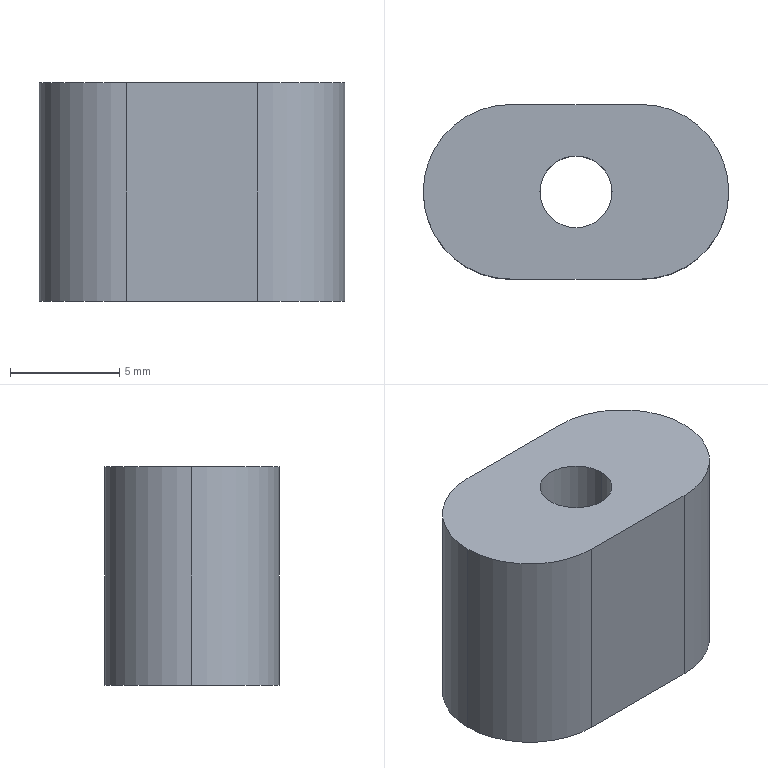Part | STEP file | 09-24 keyboard knob | 1 solid | 10 faces | box 14 x 8 x 10 mm | volume 897.125 mm3 | cylinder 6 | plane 4 | commonest cylinder face diameters 8 x4 3.3 x2
STEP:
#1=CARTESIAN_POINT('',(-1.65,0.,0.));
#2=VERTEX_POINT('',#1);
#3=CARTESIAN_POINT('',(1.65,0.,0.));
#4=VERTEX_POINT('',#3);
#5=CARTESIAN_POINT('',(0.,0.,0.));
#6=DIRECTION('',(0.,0.,1.));
#7=DIRECTION('',(1.,0.,0.));
#8=AXIS2_PLACEMENT_3D('',#5,#6,#7);
#9=CIRCLE('',#8,1.65);
#10=EDGE_CURVE('',#2,#4,#9,.T.);
#11=ORIENTED_EDGE('',*,*,#10,.F.);
#12=CARTESIAN_POINT('',(-1.65,0.,10.));
#13=VERTEX_POINT('',#12);
#14=CARTESIAN_POINT('',(-1.65,0.,10.));
#15=DIRECTION('',(0.,0.,1.));
#16=VECTOR('',#15,1000.);
#17=LINE('',#14,#16);
#18=EDGE_CURVE('',#2,#13,#17,.T.);
#19=ORIENTED_EDGE('',*,*,#18,.T.);
#20=CARTESIAN_POINT('',(1.65,0.,10.));
#21=VERTEX_POINT('',#20);
#22=CARTESIAN_POINT('',(0.,0.,10.));
#23=DIRECTION('',(0.,0.,1.));
#24=DIRECTION('',(1.,0.,0.));
#25=AXIS2_PLACEMENT_3D('',#22,#23,#24);
#26=CIRCLE('',#25,1.65);
#27=EDGE_CURVE('',#13,#21,#26,.T.);
#28=ORIENTED_EDGE('',*,*,#27,.T.);
#29=CARTESIAN_POINT('',(1.65,0.,10.));
#30=DIRECTION('',(0.,0.,1.));
#31=VECTOR('',#30,1000.);
#32=LINE('',#29,#31);
#33=EDGE_CURVE('',#4,#21,#32,.T.);
#34=ORIENTED_EDGE('',*,*,#33,.F.);
#35=EDGE_LOOP('',(#11,#19,#28,#34));
#36=FACE_OUTER_BOUND('',#35,.T.);
#37=CARTESIAN_POINT('',(0.,0.,10.));
#38=DIRECTION('',(0.,0.,1.));
#39=DIRECTION('',(1.,0.,0.));
#40=AXIS2_PLACEMENT_3D('',#37,#38,#39);
#41=CYLINDRICAL_SURFACE('',#40,1.65);
#42=ADVANCED_FACE('',(#36),#41,.F.);
#43=CARTESIAN_POINT('',(3.,4.,10.));
#44=VERTEX_POINT('',#43);
#45=CARTESIAN_POINT('',(-3.,4.,10.));
#46=VERTEX_POINT('',#45);
#47=CARTESIAN_POINT('',(-7.,4.,10.));
#48=DIRECTION('',(-1.,0.,0.));
#49=VECTOR('',#48,1000.);
#50=LINE('',#47,#49);
#51=EDGE_CURVE('',#44,#46,#50,.T.);
#52=ORIENTED_EDGE('',*,*,#51,.F.);
#53=CARTESIAN_POINT('',(3.,4.,0.));
#54=VERTEX_POINT('',#53);
#55=CARTESIAN_POINT('',(3.,4.,10.));
#56=DIRECTION('',(0.,0.,-1.));
#57=VECTOR('',#56,1000.);
#58=LINE('',#55,#57);
#59=EDGE_CURVE('',#44,#54,#58,.T.);
#60=ORIENTED_EDGE('',*,*,#59,.T.);
#61=CARTESIAN_POINT('',(-3.,4.,0.));
#62=VERTEX_POINT('',#61);
#63=CARTESIAN_POINT('',(-7.,4.,0.));
#64=DIRECTION('',(-1.,0.,0.));
#65=VECTOR('',#64,1000.);
#66=LINE('',#63,#65);
#67=EDGE_CURVE('',#54,#62,#66,.T.);
#68=ORIENTED_EDGE('',*,*,#67,.T.);
#69=CARTESIAN_POINT('',(-3.,4.,10.));
#70=DIRECTION('',(0.,0.,1.));
#71=VECTOR('',#70,1000.);
#72=LINE('',#69,#71);
#73=EDGE_CURVE('',#62,#46,#72,.T.);
#74=ORIENTED_EDGE('',*,*,#73,.T.);
#75=EDGE_LOOP('',(#52,#60,#68,#74));
#76=FACE_OUTER_BOUND('',#75,.T.);
#77=CARTESIAN_POINT('',(-7.,4.,10.));
#78=DIRECTION('',(0.,-1.,0.));
#79=DIRECTION('',(0.,0.,-1.));
#80=AXIS2_PLACEMENT_3D('',#77,#78,#79);
#81=PLANE('',#80);
#82=ADVANCED_FACE('',(#76),#81,.F.);
#83=CARTESIAN_POINT('',(-3.,-4.,0.));
#84=VERTEX_POINT('',#83);
#85=CARTESIAN_POINT('',(3.,-4.,0.));
#86=VERTEX_POINT('',#85);
#87=CARTESIAN_POINT('',(-7.,-4.,0.));
#88=DIRECTION('',(1.,0.,0.));
#89=VECTOR('',#88,1000.);
#90=LINE('',#87,#89);
#91=EDGE_CURVE('',#84,#86,#90,.T.);
#92=ORIENTED_EDGE('',*,*,#91,.T.);
#93=CARTESIAN_POINT('',(3.,-4.,10.));
#94=VERTEX_POINT('',#93);
#95=CARTESIAN_POINT('',(3.,-4.,10.));
#96=DIRECTION('',(0.,0.,1.));
#97=VECTOR('',#96,1000.);
#98=LINE('',#95,#97);
#99=EDGE_CURVE('',#86,#94,#98,.T.);
#100=ORIENTED_EDGE('',*,*,#99,.T.);
#101=CARTESIAN_POINT('',(-3.,-4.,10.));
#102=VERTEX_POINT('',#101);
#103=CARTESIAN_POINT('',(-7.,-4.,10.));
#104=DIRECTION('',(1.,0.,0.));
#105=VECTOR('',#104,1000.);
#106=LINE('',#103,#105);
#107=EDGE_CURVE('',#102,#94,#106,.T.);
#108=ORIENTED_EDGE('',*,*,#107,.F.);
#109=CARTESIAN_POINT('',(-3.,-4.,10.));
#110=DIRECTION('',(0.,0.,-1.));
#111=VECTOR('',#110,1000.);
#112=LINE('',#109,#111);
#113=EDGE_CURVE('',#102,#84,#112,.T.);
#114=ORIENTED_EDGE('',*,*,#113,.T.);
#115=EDGE_LOOP('',(#92,#100,#108,#114));
#116=FACE_OUTER_BOUND('',#115,.T.);
#117=CARTESIAN_POINT('',(-7.,-4.,10.));
#118=DIRECTION('',(0.,1.,0.));
#119=DIRECTION('',(0.,0.,1.));
#120=AXIS2_PLACEMENT_3D('',#117,#118,#119);
#121=PLANE('',#120);
#122=ADVANCED_FACE('',(#116),#121,.F.);
#123=CARTESIAN_POINT('',(0.,0.,10.));
#124=DIRECTION('',(0.,0.,1.));
#125=DIRECTION('',(1.,0.,0.));
#126=AXIS2_PLACEMENT_3D('',#123,#124,#125);
#127=CIRCLE('',#126,1.65);
#128=EDGE_CURVE('',#21,#13,#127,.T.);
#129=ORIENTED_EDGE('',*,*,#128,.F.);
#130=ORIENTED_EDGE('',*,*,#27,.F.);
#131=EDGE_LOOP('',(#129,#130));
#132=FACE_BOUND('',#131,.T.);
#133=ORIENTED_EDGE('',*,*,#107,.T.);
#134=CARTESIAN_POINT('',(7.,0.,10.));
#135=VERTEX_POINT('',#134);
#136=CARTESIAN_POINT('',(3.,0.,10.));
#137=DIRECTION('',(0.,0.,1.));
#138=DIRECTION('',(1.,0.,0.));
#139=AXIS2_PLACEMENT_3D('',#136,#137,#138);
#140=CIRCLE('',#139,4.);
#141=EDGE_CURVE('',#94,#135,#140,.T.);
#142=ORIENTED_EDGE('',*,*,#141,.T.);
#143=CARTESIAN_POINT('',(3.,0.,10.));
#144=DIRECTION('',(0.,0.,1.));
#145=DIRECTION('',(1.,0.,0.));
#146=AXIS2_PLACEMENT_3D('',#143,#144,#145);
#147=CIRCLE('',#146,4.);
#148=EDGE_CURVE('',#135,#44,#147,.T.);
#149=ORIENTED_EDGE('',*,*,#148,.T.);
#150=ORIENTED_EDGE('',*,*,#51,.T.);
#151=CARTESIAN_POINT('',(-7.,0.,10.));
#152=VERTEX_POINT('',#151);
#153=CARTESIAN_POINT('',(-3.,0.,10.));
#154=DIRECTION('',(0.,0.,1.));
#155=DIRECTION('',(1.,0.,0.));
#156=AXIS2_PLACEMENT_3D('',#153,#154,#155);
#157=CIRCLE('',#156,4.);
#158=EDGE_CURVE('',#46,#152,#157,.T.);
#159=ORIENTED_EDGE('',*,*,#158,.T.);
#160=CARTESIAN_POINT('',(-3.,0.,10.));
#161=DIRECTION('',(0.,0.,1.));
#162=DIRECTION('',(1.,0.,0.));
#163=AXIS2_PLACEMENT_3D('',#160,#161,#162);
#164=CIRCLE('',#163,4.);
#165=EDGE_CURVE('',#152,#102,#164,.T.);
#166=ORIENTED_EDGE('',*,*,#165,.T.);
#167=EDGE_LOOP('',(#133,#142,#149,#150,#159,#166));
#168=FACE_OUTER_BOUND('',#167,.T.);
#169=CARTESIAN_POINT('',(7.,-4.,10.));
#170=DIRECTION('',(0.,0.,1.));
#171=DIRECTION('',(1.,0.,0.));
#172=AXIS2_PLACEMENT_3D('',#169,#170,#171);
#173=PLANE('',#172);
#174=ADVANCED_FACE('',(#132,#168),#173,.T.);
#175=CARTESIAN_POINT('',(0.,0.,0.));
#176=DIRECTION('',(0.,0.,1.));
#177=DIRECTION('',(1.,0.,0.));
#178=AXIS2_PLACEMENT_3D('',#175,#176,#177);
#179=CIRCLE('',#178,1.65);
#180=EDGE_CURVE('',#4,#2,#179,.T.);
#181=ORIENTED_EDGE('',*,*,#180,.T.);
#182=ORIENTED_EDGE('',*,*,#10,.T.);
#183=EDGE_LOOP('',(#181,#182));
#184=FACE_BOUND('',#183,.T.);
#185=CARTESIAN_POINT('',(7.,0.,0.));
#186=VERTEX_POINT('',#185);
#187=CARTESIAN_POINT('',(3.,0.,0.));
#188=DIRECTION('',(0.,0.,-1.));
#189=DIRECTION('',(1.,0.,0.));
#190=AXIS2_PLACEMENT_3D('',#187,#188,#189);
#191=CIRCLE('',#190,4.);
#192=EDGE_CURVE('',#54,#186,#191,.T.);
#193=ORIENTED_EDGE('',*,*,#192,.T.);
#194=CARTESIAN_POINT('',(3.,0.,0.));
#195=DIRECTION('',(0.,0.,-1.));
#196=DIRECTION('',(1.,0.,0.));
#197=AXIS2_PLACEMENT_3D('',#194,#195,#196);
#198=CIRCLE('',#197,4.);
#199=EDGE_CURVE('',#186,#86,#198,.T.);
#200=ORIENTED_EDGE('',*,*,#199,.T.);
#201=ORIENTED_EDGE('',*,*,#91,.F.);
#202=CARTESIAN_POINT('',(-7.,0.,0.));
#203=VERTEX_POINT('',#202);
#204=CARTESIAN_POINT('',(-3.,0.,0.));
#205=DIRECTION('',(0.,0.,-1.));
#206=DIRECTION('',(1.,0.,0.));
#207=AXIS2_PLACEMENT_3D('',#204,#205,#206);
#208=CIRCLE('',#207,4.);
#209=EDGE_CURVE('',#84,#203,#208,.T.);
#210=ORIENTED_EDGE('',*,*,#209,.T.);
#211=CARTESIAN_POINT('',(-3.,0.,0.));
#212=DIRECTION('',(0.,0.,-1.));
#213=DIRECTION('',(1.,0.,0.));
#214=AXIS2_PLACEMENT_3D('',#211,#212,#213);
#215=CIRCLE('',#214,4.);
#216=EDGE_CURVE('',#203,#62,#215,.T.);
#217=ORIENTED_EDGE('',*,*,#216,.T.);
#218=ORIENTED_EDGE('',*,*,#67,.F.);
#219=EDGE_LOOP('',(#193,#200,#201,#210,#217,#218));
#220=FACE_OUTER_BOUND('',#219,.T.);
#221=CARTESIAN_POINT('',(7.,-4.,0.));
#222=DIRECTION('',(0.,0.,1.));
#223=DIRECTION('',(1.,0.,0.));
#224=AXIS2_PLACEMENT_3D('',#221,#222,#223);
#225=PLANE('',#224);
#226=ADVANCED_FACE('',(#184,#220),#225,.F.);
#227=ORIENTED_EDGE('',*,*,#59,.F.);
#228=ORIENTED_EDGE('',*,*,#148,.F.);
#229=CARTESIAN_POINT('',(7.,0.,10.));
#230=DIRECTION('',(0.,0.,1.));
#231=VECTOR('',#230,1000.);
#232=LINE('',#229,#231);
#233=EDGE_CURVE('',#186,#135,#232,.T.);
#234=ORIENTED_EDGE('',*,*,#233,.F.);
#235=ORIENTED_EDGE('',*,*,#192,.F.);
#236=EDGE_LOOP('',(#227,#228,#234,#235));
#237=FACE_OUTER_BOUND('',#236,.T.);
#238=CARTESIAN_POINT('',(3.,0.,10.));
#239=DIRECTION('',(0.,0.,-1.));
#240=DIRECTION('',(-1.,0.,0.));
#241=AXIS2_PLACEMENT_3D('',#238,#239,#240);
#242=CYLINDRICAL_SURFACE('',#241,4.);
#243=ADVANCED_FACE('',(#237),#242,.T.);
#244=ORIENTED_EDGE('',*,*,#141,.F.);
#245=ORIENTED_EDGE('',*,*,#99,.F.);
#246=ORIENTED_EDGE('',*,*,#199,.F.);
#247=ORIENTED_EDGE('',*,*,#233,.T.);
#248=EDGE_LOOP('',(#244,#245,#246,#247));
#249=FACE_OUTER_BOUND('',#248,.T.);
#250=CARTESIAN_POINT('',(3.,0.,10.));
#251=DIRECTION('',(0.,0.,-1.));
#252=DIRECTION('',(-1.,0.,0.));
#253=AXIS2_PLACEMENT_3D('',#250,#251,#252);
#254=CYLINDRICAL_SURFACE('',#253,4.);
#255=ADVANCED_FACE('',(#249),#254,.T.);
#256=CARTESIAN_POINT('',(-7.,0.,10.));
#257=DIRECTION('',(0.,0.,-1.));
#258=VECTOR('',#257,1000.);
#259=LINE('',#256,#258);
#260=EDGE_CURVE('',#152,#203,#259,.T.);
#261=ORIENTED_EDGE('',*,*,#260,.F.);
#262=ORIENTED_EDGE('',*,*,#158,.F.);
#263=ORIENTED_EDGE('',*,*,#73,.F.);
#264=ORIENTED_EDGE('',*,*,#216,.F.);
#265=EDGE_LOOP('',(#261,#262,#263,#264));
#266=FACE_OUTER_BOUND('',#265,.T.);
#267=CARTESIAN_POINT('',(-3.,0.,10.));
#268=DIRECTION('',(0.,0.,-1.));
#269=DIRECTION('',(-1.,0.,0.));
#270=AXIS2_PLACEMENT_3D('',#267,#268,#269);
#271=CYLINDRICAL_SURFACE('',#270,4.);
#272=ADVANCED_FACE('',(#266),#271,.T.);
#273=ORIENTED_EDGE('',*,*,#165,.F.);
#274=ORIENTED_EDGE('',*,*,#260,.T.);
#275=ORIENTED_EDGE('',*,*,#209,.F.);
#276=ORIENTED_EDGE('',*,*,#113,.F.);
#277=EDGE_LOOP('',(#273,#274,#275,#276));
#278=FACE_OUTER_BOUND('',#277,.T.);
#279=CARTESIAN_POINT('',(-3.,0.,10.));
#280=DIRECTION('',(0.,0.,-1.));
#281=DIRECTION('',(-1.,0.,0.));
#282=AXIS2_PLACEMENT_3D('',#279,#280,#281);
#283=CYLINDRICAL_SURFACE('',#282,4.);
#284=ADVANCED_FACE('',(#278),#283,.T.);
#285=ORIENTED_EDGE('',*,*,#18,.F.);
#286=ORIENTED_EDGE('',*,*,#180,.F.);
#287=ORIENTED_EDGE('',*,*,#33,.T.);
#288=ORIENTED_EDGE('',*,*,#128,.T.);
#289=EDGE_LOOP('',(#285,#286,#287,#288));
#290=FACE_OUTER_BOUND('',#289,.T.);
#291=CARTESIAN_POINT('',(0.,0.,10.));
#292=DIRECTION('',(0.,0.,1.));
#293=DIRECTION('',(1.,0.,0.));
#294=AXIS2_PLACEMENT_3D('',#291,#292,#293);
#295=CYLINDRICAL_SURFACE('',#294,1.65);
#296=ADVANCED_FACE('',(#290),#295,.F.);
#297=CLOSED_SHELL('',(#42,#82,#122,#174,#226,#243,#255,#272,#284,#296));
#298=MANIFOLD_SOLID_BREP('',#297);
#299=CARTESIAN_POINT('',(0.,0.,0.));
#300=DIRECTION('',(0.,0.,1.));
#301=DIRECTION('',(1.,0.,0.));
#302=AXIS2_PLACEMENT_3D('',#299,#300,#301);
#303=(LENGTH_UNIT()NAMED_UNIT(*)SI_UNIT(.MILLI.,.METRE.));
#304=UNCERTAINTY_MEASURE_WITH_UNIT(LENGTH_MEASURE(0.00001),#303,'','');
#305=(NAMED_UNIT(*)PLANE_ANGLE_UNIT()SI_UNIT($,.RADIAN.));
#306=(NAMED_UNIT(*)SI_UNIT($,.STERADIAN.)SOLID_ANGLE_UNIT());
#307=(GEOMETRIC_REPRESENTATION_CONTEXT(3)GLOBAL_UNCERTAINTY_ASSIGNED_CONTEXT((#304))GLOBAL_UNIT_ASSIGNED_CONTEXT((#303,#305,#306))REPRESENTATION_CONTEXT('',''));
#308=ADVANCED_BREP_SHAPE_REPRESENTATION('',(#298,#302),#307);